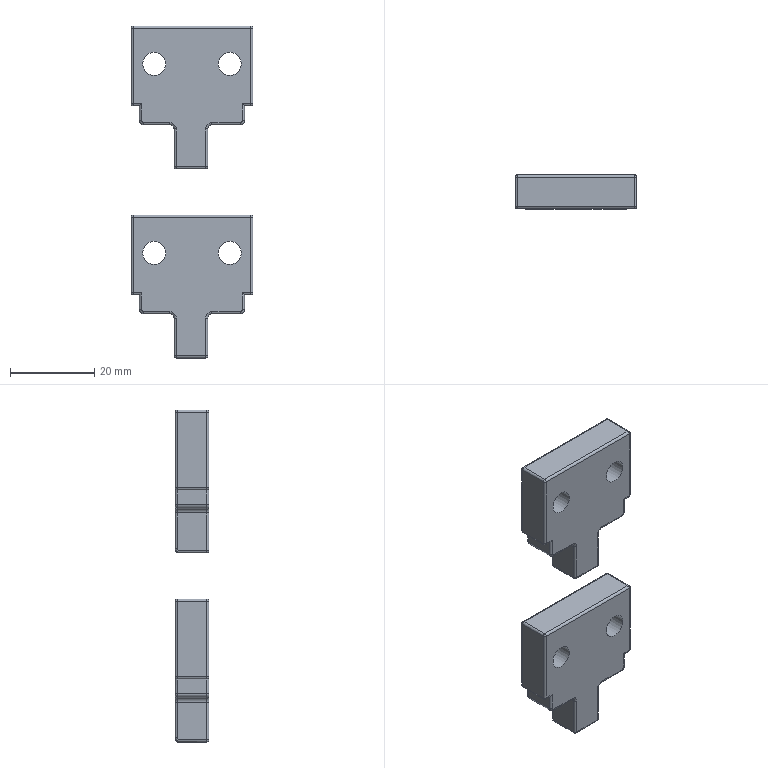CAM job | NX | 3+2 milling, drilling | part box 29 x 8 x 79 mm | stock box 30 x 10 x 84 mm
Tools:
number,name,description,diameter,corner_radius,flute_length,length,flutes
9,D10,平底铣刀-粗,10.0,0.0,35.0,75.0,2
18,D2-J,平底铣刀-精,2.0,0.0,50.0,75.0,2
7,D6-J,平底铣刀-精,6.0,0.0,25.0,75.0,2
1,D80R0.8飞刀,圆鼻刀-粗,80.0,0.8,50.0,75.0,2
1,D80R0.8飞刀-J,圆鼻刀-精,80.0,0.8,50.0,75.0,2
2,D6倒角刀,倒角刀,6.0,0.0,3.0,25.0,2
19,R1,圆球刀,2.0,1.0,6.0,50.0,2
17,钻头5.5,Twist Drill 5 mm,5.5,0.0,52.0,54.0,2
Operations:
program,operation,operation_type,tool,method,geometry_group,spindle_rpm,surface_speed,feed_per_tooth,feed_cut,feed_plunge,cut_length_mm,path_length_mm,cut_time_min,machine_time_min
B,底壁铣飞面一刀开粗_COPY,VolumeBased25DMillingOperation,D80R0.8飞刀,分层开粗-切深K-步距G,W-B,2800.0,703.696,0.5357,3000.0,100.0,748.776,1332.735,0.2496,0.308
B,底壁铣飞面一刀精光_COPY,VolumeBased25DMillingOperation,D80R0.8飞刀-J,侧刃精光-切深K-步距G,W-B,4000.0,1005.28,0.125,1000.0,100.0,186.998,222.998,0.187,0.1906
B,铣倒角_2,PlanarMilling,D6倒角刀,METHOD,W-B,8000.0,150.796,0.075,1200.0,100.0,71.178,319.397,0.0593,0.0841
B,等高螺旋爬面_COPY_COPY,ZLevelMilling,R1,等高爬面-切深K-步距G,W-B,9000.0,56.549,0.25,4500.0,100.0,7833.849,7980.643,1.741,1.756
A,顶面,FaceMilling,D80R0.8飞刀,侧刃精光-切深K-步距G,W-A,4000.0,1005.31,0.125,1000.0,100.0,173.0,209.0,0.173,0.1766
A,型腔铣开粗-中_COPY,CavityMilling,D10,分层开粗-切深K-步距G,W-A,8000.0,251.327,0.25,4000.0,100.0,10921.103,11344.413,2.73,2.794
A,打点-深0.8,Operation,D6倒角刀,NONE,W-A,8000.0,150.796,0.0312,500.0,90.0,7.2,138.467,0.0144,0.0275
A,通孔-5-6,Operation,钻头5.5,NONE,W-A,3000.0,51.836,0.025,150.0,90.0,50.609,225.286,0.3374,0.3549
A,外形侧面,ZLevelMilling,D2-J,METHOD,W-A,9000.0,56.549,0.1111,2000.0,80.0,3595.951,4066.903,1.799,1.846
A,等高螺旋爬面_COPY,ZLevelMilling,R1,等高爬面-切深K-步距G,W-A,9000.0,56.549,0.25,4500.0,100.0,6103.09,6249.539,1.356,1.371
A,铣倒角_1,PlanarMilling,D6倒角刀,METHOD,W-A,8000.0,150.796,0.0312,500.0,100.0,78.753,323.796,0.1575,0.182
A,外形半精_2,VolumeBased25DMillingOperation,D6-J,METHOD,W-A,8000.0,251.327,0.0625,1000.0,100.0,286.115,441.473,0.2861,0.3017